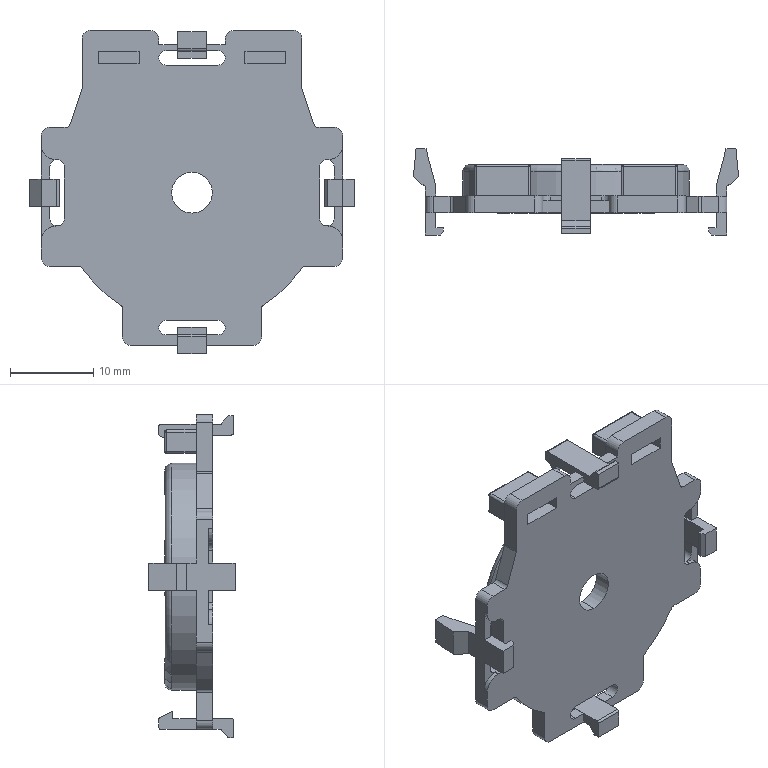Part | SolidWorks | features BaseBody 1 | 1 solid | 191 faces | box 39.14 x 10.37 x 38.9 mm | volume 2813 mm3 | plane 109 | cylinder 64 | sphere 16 | torus 2 | commonest cylinder face diameters 0.5 x24 2 x10 1 x8 1.75 x8 3.6 x6 4.9 x2